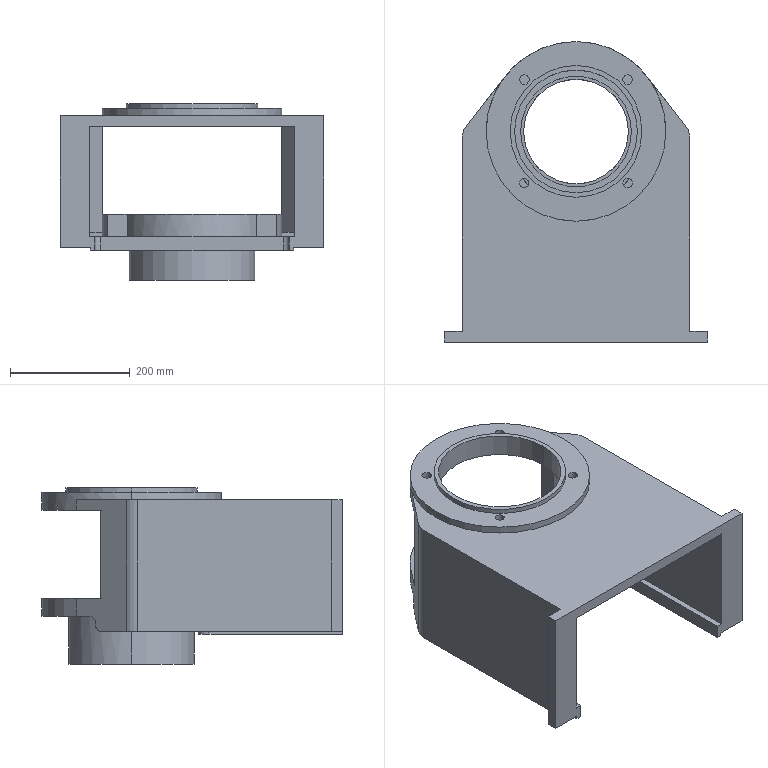Part | SolidWorks | features ICE 17, Fillet 4, HoleWzd 3, Cut 1, Extrusion 1, Revolution 1 | 1 solid | 103 faces | box 440 x 502 x 295 mm | volume 8777626 mm3 | cylinder 52 | plane 51 | commonest cylinder face diameters 18 x9 12 x8 20 x6 300 x6 16.11 x4 15.019 x2